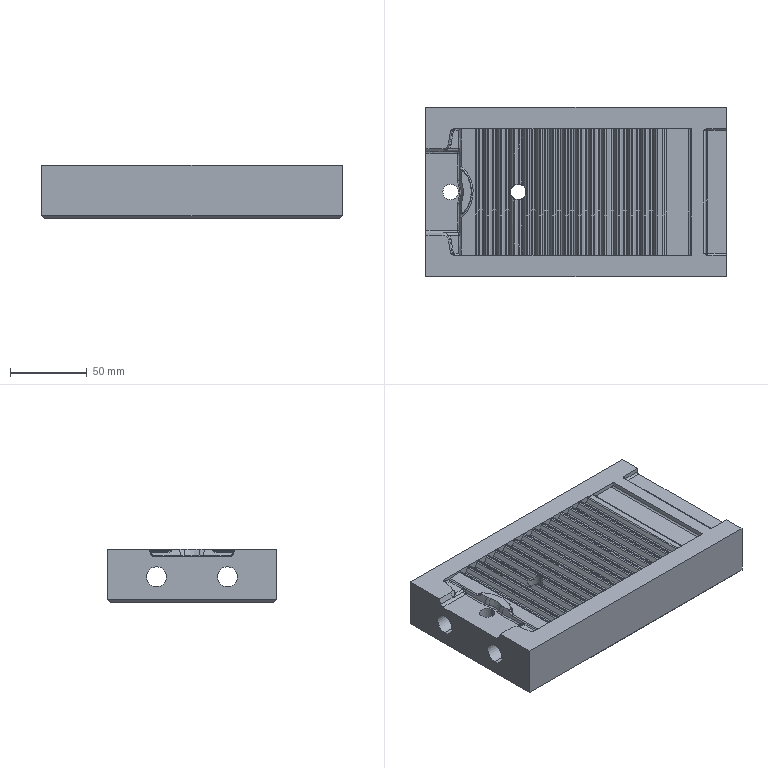Part | SolidWorks | features BaseBody 1 | 1 solid | 252 faces | box 195 x 110 x 35 mm | volume 629448 mm3 | plane 105 | cylinder 96 | spline 41 | cone 6 | torus 2 | sphere 2 | commonest cylinder face diameters 2 x64 2.4 x6 10 x6 10.5 x4 11 x4 13 x4